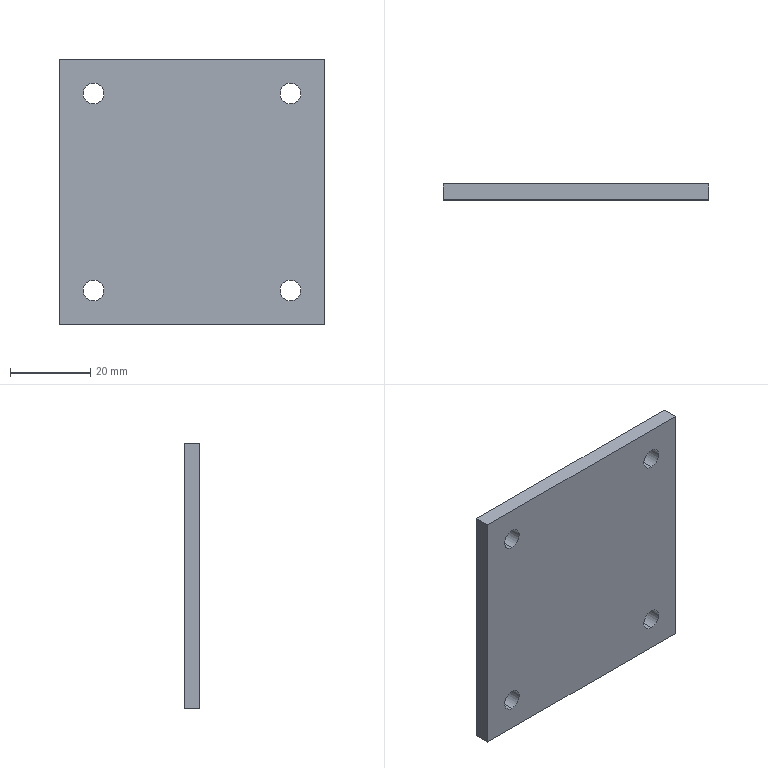Part | STEP file | 1 solid | 14 faces | box 66.15 x 3.92 x 66.15 mm | volume 16827 mm3 | cylinder 8 | plane 6 | commonest cylinder face diameters 5.145 x8
STEP:
#1=CARTESIAN_POINT('',(0.,0.,0.));
#2=DIRECTION('',(0.,0.,1.));
#3=DIRECTION('',(1.,0.,0.));
#4=AXIS2_PLACEMENT_3D('',#1,#2,#3);
#5=CARTESIAN_POINT('',(925.539,-111.474,188.835));
#6=VERTEX_POINT('',#5);
#7=CARTESIAN_POINT('',(925.539,-111.474,183.69));
#8=VERTEX_POINT('',#7);
#9=CARTESIAN_POINT('',(925.539,-111.474,186.262));
#10=DIRECTION('',(0.,1.,0.));
#11=DIRECTION('',(0.,0.,1.));
#12=AXIS2_PLACEMENT_3D('',#9,#10,#11);
#13=CIRCLE('',#12,2.572);
#14=CARTESIAN_POINT('',(925.539,-111.474,186.262));
#15=DIRECTION('',(0.,1.,0.));
#16=DIRECTION('',(0.,0.,1.));
#17=AXIS2_PLACEMENT_3D('',#14,#15,#16);
#18=CYLINDRICAL_SURFACE('',#17,2.572);
#19=CARTESIAN_POINT('',(0.,0.));
#20=DIRECTION('',(1.,0.));
#21=VECTOR('',#20,1.);
#22=LINE('',#19,#21);
#23=(GEOMETRIC_REPRESENTATION_CONTEXT(2)PARAMETRIC_REPRESENTATION_CONTEXT()REPRESENTATION_CONTEXT('',''));
#24=DEFINITIONAL_REPRESENTATION('',(#22),#23);
#25=PCURVE('',#18,#24);
#26=CARTESIAN_POINT('',(983.114,-111.474,194.837));
#27=DIRECTION('',(0.,1.,0.));
#28=DIRECTION('',(1.,0.,0.));
#29=AXIS2_PLACEMENT_3D('',#26,#27,#28);
#30=PLANE('',#29);
#31=CARTESIAN_POINT('',(-57.575,8.575));
#32=DIRECTION('',(0.,-1.));
#33=AXIS2_PLACEMENT_2D('',#31,#32);
#34=CIRCLE('',#33,2.572);
#35=(GEOMETRIC_REPRESENTATION_CONTEXT(2)PARAMETRIC_REPRESENTATION_CONTEXT()REPRESENTATION_CONTEXT('',''));
#36=DEFINITIONAL_REPRESENTATION('',(#34),#35);
#37=PCURVE('',#30,#36);
#38=SURFACE_CURVE('',#13,(#25,#37),.PCURVE_S1.);
#39=EDGE_CURVE('',#6,#8,#38,.T.);
#40=ORIENTED_EDGE('',*,*,#39,.F.);
#41=CARTESIAN_POINT('',(925.539,-115.394,188.835));
#42=VERTEX_POINT('',#41);
#43=CARTESIAN_POINT('',(925.539,-111.474,188.835));
#44=DIRECTION('',(0.,1.,0.));
#45=VECTOR('',#44,1.);
#46=LINE('',#43,#45);
#47=CARTESIAN_POINT('',(0.,0.));
#48=DIRECTION('',(0.,1.));
#49=VECTOR('',#48,1.);
#50=LINE('',#47,#49);
#51=(GEOMETRIC_REPRESENTATION_CONTEXT(2)PARAMETRIC_REPRESENTATION_CONTEXT()REPRESENTATION_CONTEXT('',''));
#52=DEFINITIONAL_REPRESENTATION('',(#50),#51);
#53=PCURVE('',#18,#52);
#54=CARTESIAN_POINT('',(925.539,-111.474,186.262));
#55=DIRECTION('',(0.,1.,0.));
#56=DIRECTION('',(0.,0.,1.));
#57=AXIS2_PLACEMENT_3D('',#54,#55,#56);
#58=CYLINDRICAL_SURFACE('',#57,2.572);
#59=CARTESIAN_POINT('',(6.283,0.));
#60=DIRECTION('',(0.,1.));
#61=VECTOR('',#60,1.);
#62=LINE('',#59,#61);
#63=(GEOMETRIC_REPRESENTATION_CONTEXT(2)PARAMETRIC_REPRESENTATION_CONTEXT()REPRESENTATION_CONTEXT('',''));
#64=DEFINITIONAL_REPRESENTATION('',(#62),#63);
#65=PCURVE('',#58,#64);
#66=SURFACE_CURVE('',#46,(#53,#65),.PCURVE_S1.);
#67=EDGE_CURVE('',#42,#6,#66,.T.);
#68=ORIENTED_EDGE('',*,*,#67,.F.);
#69=CARTESIAN_POINT('',(925.539,-115.394,183.69));
#70=VERTEX_POINT('',#69);
#71=CARTESIAN_POINT('',(925.539,-115.394,186.262));
#72=DIRECTION('',(0.,1.,0.));
#73=DIRECTION('',(0.,0.,1.));
#74=AXIS2_PLACEMENT_3D('',#71,#72,#73);
#75=CIRCLE('',#74,2.572);
#76=CARTESIAN_POINT('',(0.,-3.92));
#77=DIRECTION('',(1.,0.));
#78=VECTOR('',#77,1.);
#79=LINE('',#76,#78);
#80=(GEOMETRIC_REPRESENTATION_CONTEXT(2)PARAMETRIC_REPRESENTATION_CONTEXT()REPRESENTATION_CONTEXT('',''));
#81=DEFINITIONAL_REPRESENTATION('',(#79),#80);
#82=PCURVE('',#18,#81);
#83=CARTESIAN_POINT('',(983.114,-115.394,194.837));
#84=DIRECTION('',(0.,1.,0.));
#85=DIRECTION('',(1.,0.,0.));
#86=AXIS2_PLACEMENT_3D('',#83,#84,#85);
#87=PLANE('',#86);
#88=CARTESIAN_POINT('',(-57.575,8.575));
#89=DIRECTION('',(0.,-1.));
#90=AXIS2_PLACEMENT_2D('',#88,#89);
#91=CIRCLE('',#90,2.572);
#92=(GEOMETRIC_REPRESENTATION_CONTEXT(2)PARAMETRIC_REPRESENTATION_CONTEXT()REPRESENTATION_CONTEXT('',''));
#93=DEFINITIONAL_REPRESENTATION('',(#91),#92);
#94=PCURVE('',#87,#93);
#95=SURFACE_CURVE('',#75,(#82,#94),.PCURVE_S1.);
#96=EDGE_CURVE('',#42,#70,#95,.T.);
#97=ORIENTED_EDGE('',*,*,#96,.T.);
#98=CARTESIAN_POINT('',(925.539,-111.474,183.69));
#99=DIRECTION('',(0.,1.,0.));
#100=VECTOR('',#99,1.);
#101=LINE('',#98,#100);
#102=CARTESIAN_POINT('',(3.142,0.));
#103=DIRECTION('',(0.,1.));
#104=VECTOR('',#103,1.);
#105=LINE('',#102,#104);
#106=(GEOMETRIC_REPRESENTATION_CONTEXT(2)PARAMETRIC_REPRESENTATION_CONTEXT()REPRESENTATION_CONTEXT('',''));
#107=DEFINITIONAL_REPRESENTATION('',(#105),#106);
#108=PCURVE('',#18,#107);
#109=CARTESIAN_POINT('',(3.142,0.));
#110=DIRECTION('',(0.,1.));
#111=VECTOR('',#110,1.);
#112=LINE('',#109,#111);
#113=(GEOMETRIC_REPRESENTATION_CONTEXT(2)PARAMETRIC_REPRESENTATION_CONTEXT()REPRESENTATION_CONTEXT('',''));
#114=DEFINITIONAL_REPRESENTATION('',(#112),#113);
#115=PCURVE('',#58,#114);
#116=SURFACE_CURVE('',#101,(#108,#115),.PCURVE_S1.);
#117=EDGE_CURVE('',#70,#8,#116,.T.);
#118=ORIENTED_EDGE('',*,*,#117,.T.);
#119=EDGE_LOOP('',(#40,#68,#97,#118));
#120=FACE_BOUND('',#119,.F.);
#121=ADVANCED_FACE('',(#120),#18,.F.);
#122=CARTESIAN_POINT('',(974.539,-111.474,188.835));
#123=VERTEX_POINT('',#122);
#124=CARTESIAN_POINT('',(974.539,-111.474,183.69));
#125=VERTEX_POINT('',#124);
#126=CARTESIAN_POINT('',(974.539,-111.474,186.262));
#127=DIRECTION('',(0.,1.,0.));
#128=DIRECTION('',(0.,0.,1.));
#129=AXIS2_PLACEMENT_3D('',#126,#127,#128);
#130=CIRCLE('',#129,2.572);
#131=CARTESIAN_POINT('',(974.539,-111.474,186.262));
#132=DIRECTION('',(0.,1.,0.));
#133=DIRECTION('',(0.,0.,1.));
#134=AXIS2_PLACEMENT_3D('',#131,#132,#133);
#135=CYLINDRICAL_SURFACE('',#134,2.572);
#136=CARTESIAN_POINT('',(0.,0.));
#137=DIRECTION('',(1.,0.));
#138=VECTOR('',#137,1.);
#139=LINE('',#136,#138);
#140=(GEOMETRIC_REPRESENTATION_CONTEXT(2)PARAMETRIC_REPRESENTATION_CONTEXT()REPRESENTATION_CONTEXT('',''));
#141=DEFINITIONAL_REPRESENTATION('',(#139),#140);
#142=PCURVE('',#135,#141);
#143=CARTESIAN_POINT('',(-8.575,8.575));
#144=DIRECTION('',(0.,-1.));
#145=AXIS2_PLACEMENT_2D('',#143,#144);
#146=CIRCLE('',#145,2.572);
#147=(GEOMETRIC_REPRESENTATION_CONTEXT(2)PARAMETRIC_REPRESENTATION_CONTEXT()REPRESENTATION_CONTEXT('',''));
#148=DEFINITIONAL_REPRESENTATION('',(#146),#147);
#149=PCURVE('',#30,#148);
#150=SURFACE_CURVE('',#130,(#142,#149),.PCURVE_S1.);
#151=EDGE_CURVE('',#123,#125,#150,.T.);
#152=ORIENTED_EDGE('',*,*,#151,.F.);
#153=CARTESIAN_POINT('',(974.539,-115.394,188.835));
#154=VERTEX_POINT('',#153);
#155=CARTESIAN_POINT('',(974.539,-111.474,188.835));
#156=DIRECTION('',(0.,1.,0.));
#157=VECTOR('',#156,1.);
#158=LINE('',#155,#157);
#159=CARTESIAN_POINT('',(0.,0.));
#160=DIRECTION('',(0.,1.));
#161=VECTOR('',#160,1.);
#162=LINE('',#159,#161);
#163=(GEOMETRIC_REPRESENTATION_CONTEXT(2)PARAMETRIC_REPRESENTATION_CONTEXT()REPRESENTATION_CONTEXT('',''));
#164=DEFINITIONAL_REPRESENTATION('',(#162),#163);
#165=PCURVE('',#135,#164);
#166=CARTESIAN_POINT('',(974.539,-111.474,186.262));
#167=DIRECTION('',(0.,1.,0.));
#168=DIRECTION('',(0.,0.,1.));
#169=AXIS2_PLACEMENT_3D('',#166,#167,#168);
#170=CYLINDRICAL_SURFACE('',#169,2.572);
#171=CARTESIAN_POINT('',(6.283,0.));
#172=DIRECTION('',(0.,1.));
#173=VECTOR('',#172,1.);
#174=LINE('',#171,#173);
#175=(GEOMETRIC_REPRESENTATION_CONTEXT(2)PARAMETRIC_REPRESENTATION_CONTEXT()REPRESENTATION_CONTEXT('',''));
#176=DEFINITIONAL_REPRESENTATION('',(#174),#175);
#177=PCURVE('',#170,#176);
#178=SURFACE_CURVE('',#158,(#165,#177),.PCURVE_S1.);
#179=EDGE_CURVE('',#154,#123,#178,.T.);
#180=ORIENTED_EDGE('',*,*,#179,.F.);
#181=CARTESIAN_POINT('',(974.539,-115.394,183.69));
#182=VERTEX_POINT('',#181);
#183=CARTESIAN_POINT('',(974.539,-115.394,186.262));
#184=DIRECTION('',(0.,1.,0.));
#185=DIRECTION('',(0.,0.,1.));
#186=AXIS2_PLACEMENT_3D('',#183,#184,#185);
#187=CIRCLE('',#186,2.572);
#188=CARTESIAN_POINT('',(0.,-3.92));
#189=DIRECTION('',(1.,0.));
#190=VECTOR('',#189,1.);
#191=LINE('',#188,#190);
#192=(GEOMETRIC_REPRESENTATION_CONTEXT(2)PARAMETRIC_REPRESENTATION_CONTEXT()REPRESENTATION_CONTEXT('',''));
#193=DEFINITIONAL_REPRESENTATION('',(#191),#192);
#194=PCURVE('',#135,#193);
#195=CARTESIAN_POINT('',(-8.575,8.575));
#196=DIRECTION('',(0.,-1.));
#197=AXIS2_PLACEMENT_2D('',#195,#196);
#198=CIRCLE('',#197,2.572);
#199=(GEOMETRIC_REPRESENTATION_CONTEXT(2)PARAMETRIC_REPRESENTATION_CONTEXT()REPRESENTATION_CONTEXT('',''));
#200=DEFINITIONAL_REPRESENTATION('',(#198),#199);
#201=PCURVE('',#87,#200);
#202=SURFACE_CURVE('',#187,(#194,#201),.PCURVE_S1.);
#203=EDGE_CURVE('',#154,#182,#202,.T.);
#204=ORIENTED_EDGE('',*,*,#203,.T.);
#205=CARTESIAN_POINT('',(974.539,-111.474,183.69));
#206=DIRECTION('',(0.,1.,0.));
#207=VECTOR('',#206,1.);
#208=LINE('',#205,#207);
#209=CARTESIAN_POINT('',(3.142,0.));
#210=DIRECTION('',(0.,1.));
#211=VECTOR('',#210,1.);
#212=LINE('',#209,#211);
#213=(GEOMETRIC_REPRESENTATION_CONTEXT(2)PARAMETRIC_REPRESENTATION_CONTEXT()REPRESENTATION_CONTEXT('',''));
#214=DEFINITIONAL_REPRESENTATION('',(#212),#213);
#215=PCURVE('',#135,#214);
#216=CARTESIAN_POINT('',(3.142,0.));
#217=DIRECTION('',(0.,1.));
#218=VECTOR('',#217,1.);
#219=LINE('',#216,#218);
#220=(GEOMETRIC_REPRESENTATION_CONTEXT(2)PARAMETRIC_REPRESENTATION_CONTEXT()REPRESENTATION_CONTEXT('',''));
#221=DEFINITIONAL_REPRESENTATION('',(#219),#220);
#222=PCURVE('',#170,#221);
#223=SURFACE_CURVE('',#208,(#215,#222),.PCURVE_S1.);
#224=EDGE_CURVE('',#182,#125,#223,.T.);
#225=ORIENTED_EDGE('',*,*,#224,.T.);
#226=EDGE_LOOP('',(#152,#180,#204,#225));
#227=FACE_BOUND('',#226,.F.);
#228=ADVANCED_FACE('',(#227),#135,.F.);
#229=CARTESIAN_POINT('',(916.964,-115.394,194.837));
#230=VERTEX_POINT('',#229);
#231=CARTESIAN_POINT('',(916.964,-115.394,128.687));
#232=VERTEX_POINT('',#231);
#233=CARTESIAN_POINT('',(916.964,-115.394,194.837));
#234=DIRECTION('',(0.,0.,-1.));
#235=VECTOR('',#234,1.);
#236=LINE('',#233,#235);
#237=CARTESIAN_POINT('',(916.964,-111.474,161.762));
#238=DIRECTION('',(-1.,0.,0.));
#239=DIRECTION('',(0.,0.,1.));
#240=AXIS2_PLACEMENT_3D('',#237,#238,#239);
#241=PLANE('',#240);
#242=CARTESIAN_POINT('',(33.075,-3.92));
#243=DIRECTION('',(-1.,0.));
#244=VECTOR('',#243,1.);
#245=LINE('',#242,#244);
#246=(GEOMETRIC_REPRESENTATION_CONTEXT(2)PARAMETRIC_REPRESENTATION_CONTEXT()REPRESENTATION_CONTEXT('',''));
#247=DEFINITIONAL_REPRESENTATION('',(#245),#246);
#248=PCURVE('',#241,#247);
#249=CARTESIAN_POINT('',(-66.15,0.));
#250=DIRECTION('',(0.,1.));
#251=VECTOR('',#250,1.);
#252=LINE('',#249,#251);
#253=(GEOMETRIC_REPRESENTATION_CONTEXT(2)PARAMETRIC_REPRESENTATION_CONTEXT()REPRESENTATION_CONTEXT('',''));
#254=DEFINITIONAL_REPRESENTATION('',(#252),#253);
#255=PCURVE('',#87,#254);
#256=SURFACE_CURVE('',#236,(#248,#255),.PCURVE_S1.);
#257=EDGE_CURVE('',#230,#232,#256,.T.);
#258=ORIENTED_EDGE('',*,*,#257,.F.);
#259=CARTESIAN_POINT('',(916.964,-111.474,194.837));
#260=VERTEX_POINT('',#259);
#261=CARTESIAN_POINT('',(916.964,-115.394,194.837));
#262=DIRECTION('',(0.,1.,0.));
#263=VECTOR('',#262,1.);
#264=LINE('',#261,#263);
#265=CARTESIAN_POINT('',(33.075,-3.92));
#266=DIRECTION('',(0.,1.));
#267=VECTOR('',#266,1.);
#268=LINE('',#265,#267);
#269=(GEOMETRIC_REPRESENTATION_CONTEXT(2)PARAMETRIC_REPRESENTATION_CONTEXT()REPRESENTATION_CONTEXT('',''));
#270=DEFINITIONAL_REPRESENTATION('',(#268),#269);
#271=PCURVE('',#241,#270);
#272=CARTESIAN_POINT('',(983.114,-115.394,194.837));
#273=DIRECTION('',(0.,0.,1.));
#274=DIRECTION('',(1.,0.,0.));
#275=AXIS2_PLACEMENT_3D('',#272,#273,#274);
#276=PLANE('',#275);
#277=CARTESIAN_POINT('',(-66.15,0.));
#278=DIRECTION('',(0.,1.));
#279=VECTOR('',#278,1.);
#280=LINE('',#277,#279);
#281=(GEOMETRIC_REPRESENTATION_CONTEXT(2)PARAMETRIC_REPRESENTATION_CONTEXT()REPRESENTATION_CONTEXT('',''));
#282=DEFINITIONAL_REPRESENTATION('',(#280),#281);
#283=PCURVE('',#276,#282);
#284=SURFACE_CURVE('',#264,(#271,#283),.PCURVE_S1.);
#285=EDGE_CURVE('',#230,#260,#284,.T.);
#286=ORIENTED_EDGE('',*,*,#285,.T.);
#287=CARTESIAN_POINT('',(916.964,-111.474,128.687));
#288=VERTEX_POINT('',#287);
#289=CARTESIAN_POINT('',(916.964,-111.474,194.837));
#290=DIRECTION('',(0.,0.,-1.));
#291=VECTOR('',#290,1.);
#292=LINE('',#289,#291);
#293=CARTESIAN_POINT('',(33.075,0.));
#294=DIRECTION('',(-1.,0.));
#295=VECTOR('',#294,1.);
#296=LINE('',#293,#295);
#297=(GEOMETRIC_REPRESENTATION_CONTEXT(2)PARAMETRIC_REPRESENTATION_CONTEXT()REPRESENTATION_CONTEXT('',''));
#298=DEFINITIONAL_REPRESENTATION('',(#296),#297);
#299=PCURVE('',#241,#298);
#300=CARTESIAN_POINT('',(-66.15,0.));
#301=DIRECTION('',(0.,1.));
#302=VECTOR('',#301,1.);
#303=LINE('',#300,#302);
#304=(GEOMETRIC_REPRESENTATION_CONTEXT(2)PARAMETRIC_REPRESENTATION_CONTEXT()REPRESENTATION_CONTEXT('',''));
#305=DEFINITIONAL_REPRESENTATION('',(#303),#304);
#306=PCURVE('',#30,#305);
#307=SURFACE_CURVE('',#292,(#299,#306),.PCURVE_S1.);
#308=EDGE_CURVE('',#260,#288,#307,.T.);
#309=ORIENTED_EDGE('',*,*,#308,.T.);
#310=CARTESIAN_POINT('',(916.964,-111.474,128.687));
#311=DIRECTION('',(0.,-1.,0.));
#312=VECTOR('',#311,1.);
#313=LINE('',#310,#312);
#314=CARTESIAN_POINT('',(-33.075,0.));
#315=DIRECTION('',(0.,-1.));
#316=VECTOR('',#315,1.);
#317=LINE('',#314,#316);
#318=(GEOMETRIC_REPRESENTATION_CONTEXT(2)PARAMETRIC_REPRESENTATION_CONTEXT()REPRESENTATION_CONTEXT('',''));
#319=DEFINITIONAL_REPRESENTATION('',(#317),#318);
#320=PCURVE('',#241,#319);
#321=CARTESIAN_POINT('',(983.114,-111.474,128.687));
#322=DIRECTION('',(0.,0.,-1.));
#323=DIRECTION('',(0.,-1.,0.));
#324=AXIS2_PLACEMENT_3D('',#321,#322,#323);
#325=PLANE('',#324);
#326=CARTESIAN_POINT('',(0.,66.15));
#327=DIRECTION('',(1.,0.));
#328=VECTOR('',#327,1.);
#329=LINE('',#326,#328);
#330=(GEOMETRIC_REPRESENTATION_CONTEXT(2)PARAMETRIC_REPRESENTATION_CONTEXT()REPRESENTATION_CONTEXT('',''));
#331=DEFINITIONAL_REPRESENTATION('',(#329),#330);
#332=PCURVE('',#325,#331);
#333=SURFACE_CURVE('',#313,(#320,#332),.PCURVE_S1.);
#334=EDGE_CURVE('',#288,#232,#333,.T.);
#335=ORIENTED_EDGE('',*,*,#334,.T.);
#336=EDGE_LOOP('',(#258,#286,#309,#335));
#337=FACE_BOUND('',#336,.T.);
#338=ADVANCED_FACE('',(#337),#241,.T.);
#339=CARTESIAN_POINT('',(983.114,-115.394,194.837));
#340=VERTEX_POINT('',#339);
#341=CARTESIAN_POINT('',(983.114,-115.394,128.687));
#342=VERTEX_POINT('',#341);
#343=CARTESIAN_POINT('',(983.114,-115.394,194.837));
#344=DIRECTION('',(0.,0.,-1.));
#345=VECTOR('',#344,1.);
#346=LINE('',#343,#345);
#347=CARTESIAN_POINT('',(983.114,-111.474,161.762));
#348=DIRECTION('',(-1.,0.,0.));
#349=DIRECTION('',(0.,0.,1.));
#350=AXIS2_PLACEMENT_3D('',#347,#348,#349);
#351=PLANE('',#350);
#352=CARTESIAN_POINT('',(33.075,-3.92));
#353=DIRECTION('',(-1.,0.));
#354=VECTOR('',#353,1.);
#355=LINE('',#352,#354);
#356=(GEOMETRIC_REPRESENTATION_CONTEXT(2)PARAMETRIC_REPRESENTATION_CONTEXT()REPRESENTATION_CONTEXT('',''));
#357=DEFINITIONAL_REPRESENTATION('',(#355),#356);
#358=PCURVE('',#351,#357);
#359=CARTESIAN_POINT('',(0.,0.));
#360=DIRECTION('',(0.,1.));
#361=VECTOR('',#360,1.);
#362=LINE('',#359,#361);
#363=(GEOMETRIC_REPRESENTATION_CONTEXT(2)PARAMETRIC_REPRESENTATION_CONTEXT()REPRESENTATION_CONTEXT('',''));
#364=DEFINITIONAL_REPRESENTATION('',(#362),#363);
#365=PCURVE('',#87,#364);
#366=SURFACE_CURVE('',#346,(#358,#365),.PCURVE_S1.);
#367=EDGE_CURVE('',#340,#342,#366,.T.);
#368=ORIENTED_EDGE('',*,*,#367,.T.);
#369=CARTESIAN_POINT('',(983.114,-111.474,128.687));
#370=VERTEX_POINT('',#369);
#371=CARTESIAN_POINT('',(983.114,-111.474,128.687));
#372=DIRECTION('',(0.,-1.,0.));
#373=VECTOR('',#372,1.);
#374=LINE('',#371,#373);
#375=CARTESIAN_POINT('',(-33.075,0.));
#376=DIRECTION('',(0.,-1.));
#377=VECTOR('',#376,1.);
#378=LINE('',#375,#377);
#379=(GEOMETRIC_REPRESENTATION_CONTEXT(2)PARAMETRIC_REPRESENTATION_CONTEXT()REPRESENTATION_CONTEXT('',''));
#380=DEFINITIONAL_REPRESENTATION('',(#378),#379);
#381=PCURVE('',#351,#380);
#382=CARTESIAN_POINT('',(0.,0.));
#383=DIRECTION('',(1.,0.));
#384=VECTOR('',#383,1.);
#385=LINE('',#382,#384);
#386=(GEOMETRIC_REPRESENTATION_CONTEXT(2)PARAMETRIC_REPRESENTATION_CONTEXT()REPRESENTATION_CONTEXT('',''));
#387=DEFINITIONAL_REPRESENTATION('',(#385),#386);
#388=PCURVE('',#325,#387);
#389=SURFACE_CURVE('',#374,(#381,#388),.PCURVE_S1.);
#390=EDGE_CURVE('',#370,#342,#389,.T.);
#391=ORIENTED_EDGE('',*,*,#390,.F.);
#392=CARTESIAN_POINT('',(983.114,-111.474,194.837));
#393=VERTEX_POINT('',#392);
#394=CARTESIAN_POINT('',(983.114,-111.474,194.837));
#395=DIRECTION('',(0.,0.,-1.));
#396=VECTOR('',#395,1.);
#397=LINE('',#394,#396);
#398=CARTESIAN_POINT('',(33.075,0.));
#399=DIRECTION('',(-1.,0.));
#400=VECTOR('',#399,1.);
#401=LINE('',#398,#400);
#402=(GEOMETRIC_REPRESENTATION_CONTEXT(2)PARAMETRIC_REPRESENTATION_CONTEXT()REPRESENTATION_CONTEXT('',''));
#403=DEFINITIONAL_REPRESENTATION('',(#401),#402);
#404=PCURVE('',#351,#403);
#405=CARTESIAN_POINT('',(0.,0.));
#406=DIRECTION('',(0.,1.));
#407=VECTOR('',#406,1.);
#408=LINE('',#405,#407);
#409=(GEOMETRIC_REPRESENTATION_CONTEXT(2)PARAMETRIC_REPRESENTATION_CONTEXT()REPRESENTATION_CONTEXT('',''));
#410=DEFINITIONAL_REPRESENTATION('',(#408),#409);
#411=PCURVE('',#30,#410);
#412=SURFACE_CURVE('',#397,(#404,#411),.PCURVE_S1.);
#413=EDGE_CURVE('',#393,#370,#412,.T.);
#414=ORIENTED_EDGE('',*,*,#413,.F.);
#415=CARTESIAN_POINT('',(983.114,-115.394,194.837));
#416=DIRECTION('',(0.,1.,0.));
#417=VECTOR('',#416,1.);
#418=LINE('',#415,#417);
#419=CARTESIAN_POINT('',(33.075,-3.92));
#420=DIRECTION('',(0.,1.));
#421=VECTOR('',#420,1.);
#422=LINE('',#419,#421);
#423=(GEOMETRIC_REPRESENTATION_CONTEXT(2)PARAMETRIC_REPRESENTATION_CONTEXT()REPRESENTATION_CONTEXT('',''));
#424=DEFINITIONAL_REPRESENTATION('',(#422),#423);
#425=PCURVE('',#351,#424);
#426=CARTESIAN_POINT('',(0.,0.));
#427=DIRECTION('',(0.,1.));
#428=VECTOR('',#427,1.);
#429=LINE('',#426,#428);
#430=(GEOMETRIC_REPRESENTATION_CONTEXT(2)PARAMETRIC_REPRESENTATION_CONTEXT()REPRESENTATION_CONTEXT('',''));
#431=DEFINITIONAL_REPRESENTATION('',(#429),#430);
#432=PCURVE('',#276,#431);
#433=SURFACE_CURVE('',#418,(#425,#432),.PCURVE_S1.);
#434=EDGE_CURVE('',#340,#393,#433,.T.);
#435=ORIENTED_EDGE('',*,*,#434,.F.);
#436=EDGE_LOOP('',(#368,#391,#414,#435));
#437=FACE_BOUND('',#436,.T.);
#438=ADVANCED_FACE('',(#437),#351,.F.);
#439=ORIENTED_EDGE('',*,*,#285,.F.);
#440=CARTESIAN_POINT('',(983.114,-115.394,194.837));
#441=DIRECTION('',(-1.,0.,0.));
#442=VECTOR('',#441,1.);
#443=LINE('',#440,#442);
#444=CARTESIAN_POINT('',(0.,0.));
#445=DIRECTION('',(-1.,0.));
#446=VECTOR('',#445,1.);
#447=LINE('',#444,#446);
#448=(GEOMETRIC_REPRESENTATION_CONTEXT(2)PARAMETRIC_REPRESENTATION_CONTEXT()REPRESENTATION_CONTEXT('',''));
#449=DEFINITIONAL_REPRESENTATION('',(#447),#448);
#450=PCURVE('',#276,#449);
#451=CARTESIAN_POINT('',(0.,0.));
#452=DIRECTION('',(-1.,0.));
#453=VECTOR('',#452,1.);
#454=LINE('',#451,#453);
#455=(GEOMETRIC_REPRESENTATION_CONTEXT(2)PARAMETRIC_REPRESENTATION_CONTEXT()REPRESENTATION_CONTEXT('',''));
#456=DEFINITIONAL_REPRESENTATION('',(#454),#455);
#457=PCURVE('',#87,#456);
#458=SURFACE_CURVE('',#443,(#450,#457),.PCURVE_S1.);
#459=EDGE_CURVE('',#340,#230,#458,.T.);
#460=ORIENTED_EDGE('',*,*,#459,.F.);
#461=ORIENTED_EDGE('',*,*,#434,.T.);
#462=CARTESIAN_POINT('',(983.114,-111.474,194.837));
#463=DIRECTION('',(-1.,0.,0.));
#464=VECTOR('',#463,1.);
#465=LINE('',#462,#464);
#466=CARTESIAN_POINT('',(0.,3.92));
#467=DIRECTION('',(-1.,0.));
#468=VECTOR('',#467,1.);
#469=LINE('',#466,#468);
#470=(GEOMETRIC_REPRESENTATION_CONTEXT(2)PARAMETRIC_REPRESENTATION_CONTEXT()REPRESENTATION_CONTEXT('',''));
#471=DEFINITIONAL_REPRESENTATION('',(#469),#470);
#472=PCURVE('',#276,#471);
#473=CARTESIAN_POINT('',(0.,0.));
#474=DIRECTION('',(-1.,0.));
#475=VECTOR('',#474,1.);
#476=LINE('',#473,#475);
#477=(GEOMETRIC_REPRESENTATION_CONTEXT(2)PARAMETRIC_REPRESENTATION_CONTEXT()REPRESENTATION_CONTEXT('',''));
#478=DEFINITIONAL_REPRESENTATION('',(#476),#477);
#479=PCURVE('',#30,#478);
#480=SURFACE_CURVE('',#465,(#472,#479),.PCURVE_S1.);
#481=EDGE_CURVE('',#393,#260,#480,.T.);
#482=ORIENTED_EDGE('',*,*,#481,.T.);
#483=EDGE_LOOP('',(#439,#460,#461,#482));
#484=FACE_BOUND('',#483,.T.);
#485=ADVANCED_FACE('',(#484),#276,.T.);
#486=CARTESIAN_POINT('',(925.539,-111.474,139.835));
#487=VERTEX_POINT('',#486);
#488=CARTESIAN_POINT('',(925.539,-111.474,134.69));
#489=VERTEX_POINT('',#488);
#490=CARTESIAN_POINT('',(925.539,-111.474,137.262));
#491=DIRECTION('',(0.,1.,0.));
#492=DIRECTION('',(0.,0.,1.));
#493=AXIS2_PLACEMENT_3D('',#490,#491,#492);
#494=CIRCLE('',#493,2.572);
#495=CARTESIAN_POINT('',(-57.575,57.575));
#496=DIRECTION('',(0.,-1.));
#497=AXIS2_PLACEMENT_2D('',#495,#496);
#498=CIRCLE('',#497,2.572);
#499=(GEOMETRIC_REPRESENTATION_CONTEXT(2)PARAMETRIC_REPRESENTATION_CONTEXT()REPRESENTATION_CONTEXT('',''));
#500=DEFINITIONAL_REPRESENTATION('',(#498),#499);
#501=PCURVE('',#30,#500);
#502=CARTESIAN_POINT('',(925.539,-111.474,137.262));
#503=DIRECTION('',(0.,1.,0.));
#504=DIRECTION('',(0.,0.,1.));
#505=AXIS2_PLACEMENT_3D('',#502,#503,#504);
#506=CYLINDRICAL_SURFACE('',#505,2.572);
#507=CARTESIAN_POINT('',(0.,0.));
#508=DIRECTION('',(1.,0.));
#509=VECTOR('',#508,1.);
#510=LINE('',#507,#509);
#511=(GEOMETRIC_REPRESENTATION_CONTEXT(2)PARAMETRIC_REPRESENTATION_CONTEXT()REPRESENTATION_CONTEXT('',''));
#512=DEFINITIONAL_REPRESENTATION('',(#510),#511);
#513=PCURVE('',#506,#512);
#514=SURFACE_CURVE('',#494,(#501,#513),.PCURVE_S1.);
#515=EDGE_CURVE('',#487,#489,#514,.T.);
#516=ORIENTED_EDGE('',*,*,#515,.F.);
#517=CARTESIAN_POINT('',(925.539,-111.474,137.262));
#518=DIRECTION('',(0.,1.,0.));
#519=DIRECTION('',(0.,0.,1.));
#520=AXIS2_PLACEMENT_3D('',#517,#518,#519);
#521=CIRCLE('',#520,2.572);
#522=CARTESIAN_POINT('',(-57.575,57.575));
#523=DIRECTION('',(0.,-1.));
#524=AXIS2_PLACEMENT_2D('',#522,#523);
#525=CIRCLE('',#524,2.572);
#526=(GEOMETRIC_REPRESENTATION_CONTEXT(2)PARAMETRIC_REPRESENTATION_CONTEXT()REPRESENTATION_CONTEXT('',''));
#527=DEFINITIONAL_REPRESENTATION('',(#525),#526);
#528=PCURVE('',#30,#527);
#529=CARTESIAN_POINT('',(925.539,-111.474,137.262));
#530=DIRECTION('',(0.,1.,0.));
#531=DIRECTION('',(0.,0.,1.));
#532=AXIS2_PLACEMENT_3D('',#529,#530,#531);
#533=CYLINDRICAL_SURFACE('',#532,2.572);
#534=CARTESIAN_POINT('',(0.,0.));
#535=DIRECTION('',(1.,0.));
#536=VECTOR('',#535,1.);
#537=LINE('',#534,#536);
#538=(GEOMETRIC_REPRESENTATION_CONTEXT(2)PARAMETRIC_REPRESENTATION_CONTEXT()REPRESENTATION_CONTEXT('',''));
#539=DEFINITIONAL_REPRESENTATION('',(#537),#538);
#540=PCURVE('',#533,#539);
#541=SURFACE_CURVE('',#521,(#528,#540),.PCURVE_S1.);
#542=EDGE_CURVE('',#489,#487,#541,.T.);
#543=ORIENTED_EDGE('',*,*,#542,.F.);
#544=EDGE_LOOP('',(#516,#543));
#545=FACE_BOUND('',#544,.T.);
#546=CARTESIAN_POINT('',(974.539,-111.474,139.835));
#547=VERTEX_POINT('',#546);
#548=CARTESIAN_POINT('',(974.539,-111.474,134.69));
#549=VERTEX_POINT('',#548);
#550=CARTESIAN_POINT('',(974.539,-111.474,137.262));
#551=DIRECTION('',(0.,1.,0.));
#552=DIRECTION('',(0.,0.,1.));
#553=AXIS2_PLACEMENT_3D('',#550,#551,#552);
#554=CIRCLE('',#553,2.572);
#555=CARTESIAN_POINT('',(-8.575,57.575));
#556=DIRECTION('',(0.,-1.));
#557=AXIS2_PLACEMENT_2D('',#555,#556);
#558=CIRCLE('',#557,2.572);
#559=(GEOMETRIC_REPRESENTATION_CONTEXT(2)PARAMETRIC_REPRESENTATION_CONTEXT()REPRESENTATION_CONTEXT('',''));
#560=DEFINITIONAL_REPRESENTATION('',(#558),#559);
#561=PCURVE('',#30,#560);
#562=CARTESIAN_POINT('',(974.539,-111.474,137.262));
#563=DIRECTION('',(0.,1.,0.));
#564=DIRECTION('',(0.,0.,1.));
#565=AXIS2_PLACEMENT_3D('',#562,#563,#564);
#566=CYLINDRICAL_SURFACE('',#565,2.572);
#567=CARTESIAN_POINT('',(0.,0.));
#568=DIRECTION('',(1.,0.));
#569=VECTOR('',#568,1.);
#570=LINE('',#567,#569);
#571=(GEOMETRIC_REPRESENTATION_CONTEXT(2)PARAMETRIC_REPRESENTATION_CONTEXT()REPRESENTATION_CONTEXT('',''));
#572=DEFINITIONAL_REPRESENTATION('',(#570),#571);
#573=PCURVE('',#566,#572);
#574=SURFACE_CURVE('',#554,(#561,#573),.PCURVE_S1.);
#575=EDGE_CURVE('',#547,#549,#574,.T.);
#576=ORIENTED_EDGE('',*,*,#575,.F.);
#577=CARTESIAN_POINT('',(974.539,-111.474,137.262));
#578=DIRECTION('',(0.,1.,0.));
#579=DIRECTION('',(0.,0.,1.));
#580=AXIS2_PLACEMENT_3D('',#577,#578,#579);
#581=CIRCLE('',#580,2.572);
#582=CARTESIAN_POINT('',(-8.575,57.575));
#583=DIRECTION('',(0.,-1.));
#584=AXIS2_PLACEMENT_2D('',#582,#583);
#585=CIRCLE('',#584,2.572);
#586=(GEOMETRIC_REPRESENTATION_CONTEXT(2)PARAMETRIC_REPRESENTATION_CONTEXT()REPRESENTATION_CONTEXT('',''));
#587=DEFINITIONAL_REPRESENTATION('',(#585),#586);
#588=PCURVE('',#30,#587);
#589=CARTESIAN_POINT('',(974.539,-111.474,137.262));
#590=DIRECTION('',(0.,1.,0.));
#591=DIRECTION('',(0.,0.,1.));
#592=AXIS2_PLACEMENT_3D('',#589,#590,#591);
#593=CYLINDRICAL_SURFACE('',#592,2.572);
#594=CARTESIAN_POINT('',(0.,0.));
#595=DIRECTION('',(1.,0.));
#596=VECTOR('',#595,1.);
#597=LINE('',#594,#596);
#598=(GEOMETRIC_REPRESENTATION_CONTEXT(2)PARAMETRIC_REPRESENTATION_CONTEXT()REPRESENTATION_CONTEXT('',''));
#599=DEFINITIONAL_REPRESENTATION('',(#597),#598);
#600=PCURVE('',#593,#599);
#601=SURFACE_CURVE('',#581,(#588,#600),.PCURVE_S1.);
#602=EDGE_CURVE('',#549,#547,#601,.T.);
#603=ORIENTED_EDGE('',*,*,#602,.F.);
#604=EDGE_LOOP('',(#576,#603));
#605=FACE_BOUND('',#604,.T.);
#606=ORIENTED_EDGE('',*,*,#151,.F.);
#607=CARTESIAN_POINT('',(974.539,-111.474,186.262));
#608=DIRECTION('',(0.,1.,0.));
#609=DIRECTION('',(0.,0.,1.));
#610=AXIS2_PLACEMENT_3D('',#607,#608,#609);
#611=CIRCLE('',#610,2.572);
#612=CARTESIAN_POINT('',(-8.575,8.575));
#613=DIRECTION('',(0.,-1.));
#614=AXIS2_PLACEMENT_2D('',#612,#613);
#615=CIRCLE('',#614,2.572);
#616=(GEOMETRIC_REPRESENTATION_CONTEXT(2)PARAMETRIC_REPRESENTATION_CONTEXT()REPRESENTATION_CONTEXT('',''));
#617=DEFINITIONAL_REPRESENTATION('',(#615),#616);
#618=PCURVE('',#30,#617);
#619=CARTESIAN_POINT('',(0.,0.));
#620=DIRECTION('',(1.,0.));
#621=VECTOR('',#620,1.);
#622=LINE('',#619,#621);
#623=(GEOMETRIC_REPRESENTATION_CONTEXT(2)PARAMETRIC_REPRESENTATION_CONTEXT()REPRESENTATION_CONTEXT('',''));
#624=DEFINITIONAL_REPRESENTATION('',(#622),#623);
#625=PCURVE('',#170,#624);
#626=SURFACE_CURVE('',#611,(#618,#625),.PCURVE_S1.);
#627=EDGE_CURVE('',#125,#123,#626,.T.);
#628=ORIENTED_EDGE('',*,*,#627,.F.);
#629=EDGE_LOOP('',(#606,#628));
#630=FACE_BOUND('',#629,.T.);
#631=ORIENTED_EDGE('',*,*,#39,.F.);
#632=CARTESIAN_POINT('',(925.539,-111.474,186.262));
#633=DIRECTION('',(0.,1.,0.));
#634=DIRECTION('',(0.,0.,1.));
#635=AXIS2_PLACEMENT_3D('',#632,#633,#634);
#636=CIRCLE('',#635,2.572);
#637=CARTESIAN_POINT('',(-57.575,8.575));
#638=DIRECTION('',(0.,-1.));
#639=AXIS2_PLACEMENT_2D('',#637,#638);
#640=CIRCLE('',#639,2.572);
#641=(GEOMETRIC_REPRESENTATION_CONTEXT(2)PARAMETRIC_REPRESENTATION_CONTEXT()REPRESENTATION_CONTEXT('',''));
#642=DEFINITIONAL_REPRESENTATION('',(#640),#641);
#643=PCURVE('',#30,#642);
#644=CARTESIAN_POINT('',(0.,0.));
#645=DIRECTION('',(1.,0.));
#646=VECTOR('',#645,1.);
#647=LINE('',#644,#646);
#648=(GEOMETRIC_REPRESENTATION_CONTEXT(2)PARAMETRIC_REPRESENTATION_CONTEXT()REPRESENTATION_CONTEXT('',''));
#649=DEFINITIONAL_REPRESENTATION('',(#647),#648);
#650=PCURVE('',#58,#649);
#651=SURFACE_CURVE('',#636,(#643,#650),.PCURVE_S1.);
#652=EDGE_CURVE('',#8,#6,#651,.T.);
#653=ORIENTED_EDGE('',*,*,#652,.F.);
#654=EDGE_LOOP('',(#631,#653));
#655=FACE_BOUND('',#654,.T.);
#656=ORIENTED_EDGE('',*,*,#308,.F.);
#657=ORIENTED_EDGE('',*,*,#481,.F.);
#658=ORIENTED_EDGE('',*,*,#413,.T.);
#659=CARTESIAN_POINT('',(983.114,-111.474,128.687));
#660=DIRECTION('',(-1.,0.,0.));
#661=VECTOR('',#660,1.);
#662=LINE('',#659,#661);
#663=CARTESIAN_POINT('',(0.,66.15));
#664=DIRECTION('',(-1.,0.));
#665=VECTOR('',#664,1.);
#666=LINE('',#663,#665);
#667=(GEOMETRIC_REPRESENTATION_CONTEXT(2)PARAMETRIC_REPRESENTATION_CONTEXT()REPRESENTATION_CONTEXT('',''));
#668=DEFINITIONAL_REPRESENTATION('',(#666),#667);
#669=PCURVE('',#30,#668);
#670=CARTESIAN_POINT('',(0.,0.));
#671=DIRECTION('',(0.,1.));
#672=VECTOR('',#671,1.);
#673=LINE('',#670,#672);
#674=(GEOMETRIC_REPRESENTATION_CONTEXT(2)PARAMETRIC_REPRESENTATION_CONTEXT()REPRESENTATION_CONTEXT('',''));
#675=DEFINITIONAL_REPRESENTATION('',(#673),#674);
#676=PCURVE('',#325,#675);
#677=SURFACE_CURVE('',#662,(#669,#676),.PCURVE_S1.);
#678=EDGE_CURVE('',#370,#288,#677,.T.);
#679=ORIENTED_EDGE('',*,*,#678,.T.);
#680=EDGE_LOOP('',(#656,#657,#658,#679));
#681=FACE_BOUND('',#680,.T.);
#682=ADVANCED_FACE('',(#545,#605,#630,#655,#681),#30,.T.);
#683=ORIENTED_EDGE('',*,*,#334,.F.);
#684=ORIENTED_EDGE('',*,*,#678,.F.);
#685=ORIENTED_EDGE('',*,*,#390,.T.);
#686=CARTESIAN_POINT('',(983.114,-115.394,128.687));
#687=DIRECTION('',(-1.,0.,0.));
#688=VECTOR('',#687,1.);
#689=LINE('',#686,#688);
#690=CARTESIAN_POINT('',(3.92,0.));
#691=DIRECTION('',(0.,1.));
#692=VECTOR('',#691,1.);
#693=LINE('',#690,#692);
#694=(GEOMETRIC_REPRESENTATION_CONTEXT(2)PARAMETRIC_REPRESENTATION_CONTEXT()REPRESENTATION_CONTEXT('',''));
#695=DEFINITIONAL_REPRESENTATION('',(#693),#694);
#696=PCURVE('',#325,#695);
#697=CARTESIAN_POINT('',(0.,66.15));
#698=DIRECTION('',(-1.,0.));
#699=VECTOR('',#698,1.);
#700=LINE('',#697,#699);
#701=(GEOMETRIC_REPRESENTATION_CONTEXT(2)PARAMETRIC_REPRESENTATION_CONTEXT()REPRESENTATION_CONTEXT('',''));
#702=DEFINITIONAL_REPRESENTATION('',(#700),#701);
#703=PCURVE('',#87,#702);
#704=SURFACE_CURVE('',#689,(#696,#703),.PCURVE_S1.);
#705=EDGE_CURVE('',#342,#232,#704,.T.);
#706=ORIENTED_EDGE('',*,*,#705,.T.);
#707=EDGE_LOOP('',(#683,#684,#685,#706));
#708=FACE_BOUND('',#707,.T.);
#709=ADVANCED_FACE('',(#708),#325,.T.);
#710=CARTESIAN_POINT('',(925.539,-115.394,139.835));
#711=VERTEX_POINT('',#710);
#712=CARTESIAN_POINT('',(925.539,-115.394,134.69));
#713=VERTEX_POINT('',#712);
#714=CARTESIAN_POINT('',(925.539,-115.394,137.262));
#715=DIRECTION('',(0.,1.,0.));
#716=DIRECTION('',(0.,0.,1.));
#717=AXIS2_PLACEMENT_3D('',#714,#715,#716);
#718=CIRCLE('',#717,2.572);
#719=CARTESIAN_POINT('',(-57.575,57.575));
#720=DIRECTION('',(0.,-1.));
#721=AXIS2_PLACEMENT_2D('',#719,#720);
#722=CIRCLE('',#721,2.572);
#723=(GEOMETRIC_REPRESENTATION_CONTEXT(2)PARAMETRIC_REPRESENTATION_CONTEXT()REPRESENTATION_CONTEXT('',''));
#724=DEFINITIONAL_REPRESENTATION('',(#722),#723);
#725=PCURVE('',#87,#724);
#726=CARTESIAN_POINT('',(0.,-3.92));
#727=DIRECTION('',(1.,0.));
#728=VECTOR('',#727,1.);
#729=LINE('',#726,#728);
#730=(GEOMETRIC_REPRESENTATION_CONTEXT(2)PARAMETRIC_REPRESENTATION_CONTEXT()REPRESENTATION_CONTEXT('',''));
#731=DEFINITIONAL_REPRESENTATION('',(#729),#730);
#732=PCURVE('',#506,#731);
#733=SURFACE_CURVE('',#718,(#725,#732),.PCURVE_S1.);
#734=EDGE_CURVE('',#711,#713,#733,.T.);
#735=ORIENTED_EDGE('',*,*,#734,.T.);
#736=CARTESIAN_POINT('',(925.539,-115.394,137.262));
#737=DIRECTION('',(0.,1.,0.));
#738=DIRECTION('',(0.,0.,1.));
#739=AXIS2_PLACEMENT_3D('',#736,#737,#738);
#740=CIRCLE('',#739,2.572);
#741=CARTESIAN_POINT('',(-57.575,57.575));
#742=DIRECTION('',(0.,-1.));
#743=AXIS2_PLACEMENT_2D('',#741,#742);
#744=CIRCLE('',#743,2.572);
#745=(GEOMETRIC_REPRESENTATION_CONTEXT(2)PARAMETRIC_REPRESENTATION_CONTEXT()REPRESENTATION_CONTEXT('',''));
#746=DEFINITIONAL_REPRESENTATION('',(#744),#745);
#747=PCURVE('',#87,#746);
#748=CARTESIAN_POINT('',(0.,-3.92));
#749=DIRECTION('',(1.,0.));
#750=VECTOR('',#749,1.);
#751=LINE('',#748,#750);
#752=(GEOMETRIC_REPRESENTATION_CONTEXT(2)PARAMETRIC_REPRESENTATION_CONTEXT()REPRESENTATION_CONTEXT('',''));
#753=DEFINITIONAL_REPRESENTATION('',(#751),#752);
#754=PCURVE('',#533,#753);
#755=SURFACE_CURVE('',#740,(#747,#754),.PCURVE_S1.);
#756=EDGE_CURVE('',#713,#711,#755,.T.);
#757=ORIENTED_EDGE('',*,*,#756,.T.);
#758=EDGE_LOOP('',(#735,#757));
#759=FACE_BOUND('',#758,.T.);
#760=CARTESIAN_POINT('',(974.539,-115.394,139.835));
#761=VERTEX_POINT('',#760);
#762=CARTESIAN_POINT('',(974.539,-115.394,134.69));
#763=VERTEX_POINT('',#762);
#764=CARTESIAN_POINT('',(974.539,-115.394,137.262));
#765=DIRECTION('',(0.,1.,0.));
#766=DIRECTION('',(0.,0.,1.));
#767=AXIS2_PLACEMENT_3D('',#764,#765,#766);
#768=CIRCLE('',#767,2.572);
#769=CARTESIAN_POINT('',(-8.575,57.575));
#770=DIRECTION('',(0.,-1.));
#771=AXIS2_PLACEMENT_2D('',#769,#770);
#772=CIRCLE('',#771,2.572);
#773=(GEOMETRIC_REPRESENTATION_CONTEXT(2)PARAMETRIC_REPRESENTATION_CONTEXT()REPRESENTATION_CONTEXT('',''));
#774=DEFINITIONAL_REPRESENTATION('',(#772),#773);
#775=PCURVE('',#87,#774);
#776=CARTESIAN_POINT('',(0.,-3.92));
#777=DIRECTION('',(1.,0.));
#778=VECTOR('',#777,1.);
#779=LINE('',#776,#778);
#780=(GEOMETRIC_REPRESENTATION_CONTEXT(2)PARAMETRIC_REPRESENTATION_CONTEXT()REPRESENTATION_CONTEXT('',''));
#781=DEFINITIONAL_REPRESENTATION('',(#779),#780);
#782=PCURVE('',#566,#781);
#783=SURFACE_CURVE('',#768,(#775,#782),.PCURVE_S1.);
#784=EDGE_CURVE('',#761,#763,#783,.T.);
#785=ORIENTED_EDGE('',*,*,#784,.T.);
#786=CARTESIAN_POINT('',(974.539,-115.394,137.262));
#787=DIRECTION('',(0.,1.,0.));
#788=DIRECTION('',(0.,0.,1.));
#789=AXIS2_PLACEMENT_3D('',#786,#787,#788);
#790=CIRCLE('',#789,2.572);
#791=CARTESIAN_POINT('',(-8.575,57.575));
#792=DIRECTION('',(0.,-1.));
#793=AXIS2_PLACEMENT_2D('',#791,#792);
#794=CIRCLE('',#793,2.572);
#795=(GEOMETRIC_REPRESENTATION_CONTEXT(2)PARAMETRIC_REPRESENTATION_CONTEXT()REPRESENTATION_CONTEXT('',''));
#796=DEFINITIONAL_REPRESENTATION('',(#794),#795);
#797=PCURVE('',#87,#796);
#798=CARTESIAN_POINT('',(0.,-3.92));
#799=DIRECTION('',(1.,0.));
#800=VECTOR('',#799,1.);
#801=LINE('',#798,#800);
#802=(GEOMETRIC_REPRESENTATION_CONTEXT(2)PARAMETRIC_REPRESENTATION_CONTEXT()REPRESENTATION_CONTEXT('',''));
#803=DEFINITIONAL_REPRESENTATION('',(#801),#802);
#804=PCURVE('',#593,#803);
#805=SURFACE_CURVE('',#790,(#797,#804),.PCURVE_S1.);
#806=EDGE_CURVE('',#763,#761,#805,.T.);
#807=ORIENTED_EDGE('',*,*,#806,.T.);
#808=EDGE_LOOP('',(#785,#807));
#809=FACE_BOUND('',#808,.T.);
#810=ORIENTED_EDGE('',*,*,#203,.T.);
#811=CARTESIAN_POINT('',(974.539,-115.394,186.262));
#812=DIRECTION('',(0.,1.,0.));
#813=DIRECTION('',(0.,0.,1.));
#814=AXIS2_PLACEMENT_3D('',#811,#812,#813);
#815=CIRCLE('',#814,2.572);
#816=CARTESIAN_POINT('',(-8.575,8.575));
#817=DIRECTION('',(0.,-1.));
#818=AXIS2_PLACEMENT_2D('',#816,#817);
#819=CIRCLE('',#818,2.572);
#820=(GEOMETRIC_REPRESENTATION_CONTEXT(2)PARAMETRIC_REPRESENTATION_CONTEXT()REPRESENTATION_CONTEXT('',''));
#821=DEFINITIONAL_REPRESENTATION('',(#819),#820);
#822=PCURVE('',#87,#821);
#823=CARTESIAN_POINT('',(0.,-3.92));
#824=DIRECTION('',(1.,0.));
#825=VECTOR('',#824,1.);
#826=LINE('',#823,#825);
#827=(GEOMETRIC_REPRESENTATION_CONTEXT(2)PARAMETRIC_REPRESENTATION_CONTEXT()REPRESENTATION_CONTEXT('',''));
#828=DEFINITIONAL_REPRESENTATION('',(#826),#827);
#829=PCURVE('',#170,#828);
#830=SURFACE_CURVE('',#815,(#822,#829),.PCURVE_S1.);
#831=EDGE_CURVE('',#182,#154,#830,.T.);
#832=ORIENTED_EDGE('',*,*,#831,.T.);
#833=EDGE_LOOP('',(#810,#832));
#834=FACE_BOUND('',#833,.T.);
#835=ORIENTED_EDGE('',*,*,#96,.T.);
#836=CARTESIAN_POINT('',(925.539,-115.394,186.262));
#837=DIRECTION('',(0.,1.,0.));
#838=DIRECTION('',(0.,0.,1.));
#839=AXIS2_PLACEMENT_3D('',#836,#837,#838);
#840=CIRCLE('',#839,2.572);
#841=CARTESIAN_POINT('',(-57.575,8.575));
#842=DIRECTION('',(0.,-1.));
#843=AXIS2_PLACEMENT_2D('',#841,#842);
#844=CIRCLE('',#843,2.572);
#845=(GEOMETRIC_REPRESENTATION_CONTEXT(2)PARAMETRIC_REPRESENTATION_CONTEXT()REPRESENTATION_CONTEXT('',''));
#846=DEFINITIONAL_REPRESENTATION('',(#844),#845);
#847=PCURVE('',#87,#846);
#848=CARTESIAN_POINT('',(0.,-3.92));
#849=DIRECTION('',(1.,0.));
#850=VECTOR('',#849,1.);
#851=LINE('',#848,#850);
#852=(GEOMETRIC_REPRESENTATION_CONTEXT(2)PARAMETRIC_REPRESENTATION_CONTEXT()REPRESENTATION_CONTEXT('',''));
#853=DEFINITIONAL_REPRESENTATION('',(#851),#852);
#854=PCURVE('',#58,#853);
#855=SURFACE_CURVE('',#840,(#847,#854),.PCURVE_S1.);
#856=EDGE_CURVE('',#70,#42,#855,.T.);
#857=ORIENTED_EDGE('',*,*,#856,.T.);
#858=EDGE_LOOP('',(#835,#857));
#859=FACE_BOUND('',#858,.T.);
#860=ORIENTED_EDGE('',*,*,#257,.T.);
#861=ORIENTED_EDGE('',*,*,#705,.F.);
#862=ORIENTED_EDGE('',*,*,#367,.F.);
#863=ORIENTED_EDGE('',*,*,#459,.T.);
#864=EDGE_LOOP('',(#860,#861,#862,#863));
#865=FACE_BOUND('',#864,.T.);
#866=ADVANCED_FACE('',(#759,#809,#834,#859,#865),#87,.F.);
#867=ORIENTED_EDGE('',*,*,#575,.F.);
#868=CARTESIAN_POINT('',(974.539,-111.474,139.835));
#869=DIRECTION('',(0.,1.,0.));
#870=VECTOR('',#869,1.);
#871=LINE('',#868,#870);
#872=CARTESIAN_POINT('',(0.,0.));
#873=DIRECTION('',(0.,1.));
#874=VECTOR('',#873,1.);
#875=LINE('',#872,#874);
#876=(GEOMETRIC_REPRESENTATION_CONTEXT(2)PARAMETRIC_REPRESENTATION_CONTEXT()REPRESENTATION_CONTEXT('',''));
#877=DEFINITIONAL_REPRESENTATION('',(#875),#876);
#878=PCURVE('',#566,#877);
#879=CARTESIAN_POINT('',(6.283,0.));
#880=DIRECTION('',(0.,1.));
#881=VECTOR('',#880,1.);
#882=LINE('',#879,#881);
#883=(GEOMETRIC_REPRESENTATION_CONTEXT(2)PARAMETRIC_REPRESENTATION_CONTEXT()REPRESENTATION_CONTEXT('',''));
#884=DEFINITIONAL_REPRESENTATION('',(#882),#883);
#885=PCURVE('',#593,#884);
#886=SURFACE_CURVE('',#871,(#878,#885),.PCURVE_S1.);
#887=EDGE_CURVE('',#761,#547,#886,.T.);
#888=ORIENTED_EDGE('',*,*,#887,.F.);
#889=ORIENTED_EDGE('',*,*,#784,.T.);
#890=CARTESIAN_POINT('',(974.539,-111.474,134.69));
#891=DIRECTION('',(0.,1.,0.));
#892=VECTOR('',#891,1.);
#893=LINE('',#890,#892);
#894=CARTESIAN_POINT('',(3.142,0.));
#895=DIRECTION('',(0.,1.));
#896=VECTOR('',#895,1.);
#897=LINE('',#894,#896);
#898=(GEOMETRIC_REPRESENTATION_CONTEXT(2)PARAMETRIC_REPRESENTATION_CONTEXT()REPRESENTATION_CONTEXT('',''));
#899=DEFINITIONAL_REPRESENTATION('',(#897),#898);
#900=PCURVE('',#566,#899);
#901=CARTESIAN_POINT('',(3.142,0.));
#902=DIRECTION('',(0.,1.));
#903=VECTOR('',#902,1.);
#904=LINE('',#901,#903);
#905=(GEOMETRIC_REPRESENTATION_CONTEXT(2)PARAMETRIC_REPRESENTATION_CONTEXT()REPRESENTATION_CONTEXT('',''));
#906=DEFINITIONAL_REPRESENTATION('',(#904),#905);
#907=PCURVE('',#593,#906);
#908=SURFACE_CURVE('',#893,(#900,#907),.PCURVE_S1.);
#909=EDGE_CURVE('',#763,#549,#908,.T.);
#910=ORIENTED_EDGE('',*,*,#909,.T.);
#911=EDGE_LOOP('',(#867,#888,#889,#910));
#912=FACE_BOUND('',#911,.F.);
#913=ADVANCED_FACE('',(#912),#566,.F.);
#914=ORIENTED_EDGE('',*,*,#515,.F.);
#915=CARTESIAN_POINT('',(925.539,-111.474,139.835));
#916=DIRECTION('',(0.,1.,0.));
#917=VECTOR('',#916,1.);
#918=LINE('',#915,#917);
#919=CARTESIAN_POINT('',(0.,0.));
#920=DIRECTION('',(0.,1.));
#921=VECTOR('',#920,1.);
#922=LINE('',#919,#921);
#923=(GEOMETRIC_REPRESENTATION_CONTEXT(2)PARAMETRIC_REPRESENTATION_CONTEXT()REPRESENTATION_CONTEXT('',''));
#924=DEFINITIONAL_REPRESENTATION('',(#922),#923);
#925=PCURVE('',#506,#924);
#926=CARTESIAN_POINT('',(6.283,0.));
#927=DIRECTION('',(0.,1.));
#928=VECTOR('',#927,1.);
#929=LINE('',#926,#928);
#930=(GEOMETRIC_REPRESENTATION_CONTEXT(2)PARAMETRIC_REPRESENTATION_CONTEXT()REPRESENTATION_CONTEXT('',''));
#931=DEFINITIONAL_REPRESENTATION('',(#929),#930);
#932=PCURVE('',#533,#931);
#933=SURFACE_CURVE('',#918,(#925,#932),.PCURVE_S1.);
#934=EDGE_CURVE('',#711,#487,#933,.T.);
#935=ORIENTED_EDGE('',*,*,#934,.F.);
#936=ORIENTED_EDGE('',*,*,#734,.T.);
#937=CARTESIAN_POINT('',(925.539,-111.474,134.69));
#938=DIRECTION('',(0.,1.,0.));
#939=VECTOR('',#938,1.);
#940=LINE('',#937,#939);
#941=CARTESIAN_POINT('',(3.142,0.));
#942=DIRECTION('',(0.,1.));
#943=VECTOR('',#942,1.);
#944=LINE('',#941,#943);
#945=(GEOMETRIC_REPRESENTATION_CONTEXT(2)PARAMETRIC_REPRESENTATION_CONTEXT()REPRESENTATION_CONTEXT('',''));
#946=DEFINITIONAL_REPRESENTATION('',(#944),#945);
#947=PCURVE('',#506,#946);
#948=CARTESIAN_POINT('',(3.142,0.));
#949=DIRECTION('',(0.,1.));
#950=VECTOR('',#949,1.);
#951=LINE('',#948,#950);
#952=(GEOMETRIC_REPRESENTATION_CONTEXT(2)PARAMETRIC_REPRESENTATION_CONTEXT()REPRESENTATION_CONTEXT('',''));
#953=DEFINITIONAL_REPRESENTATION('',(#951),#952);
#954=PCURVE('',#533,#953);
#955=SURFACE_CURVE('',#940,(#947,#954),.PCURVE_S1.);
#956=EDGE_CURVE('',#713,#489,#955,.T.);
#957=ORIENTED_EDGE('',*,*,#956,.T.);
#958=EDGE_LOOP('',(#914,#935,#936,#957));
#959=FACE_BOUND('',#958,.F.);
#960=ADVANCED_FACE('',(#959),#506,.F.);
#961=ORIENTED_EDGE('',*,*,#934,.T.);
#962=ORIENTED_EDGE('',*,*,#542,.F.);
#963=ORIENTED_EDGE('',*,*,#956,.F.);
#964=ORIENTED_EDGE('',*,*,#756,.T.);
#965=EDGE_LOOP('',(#961,#962,#963,#964));
#966=FACE_BOUND('',#965,.F.);
#967=ADVANCED_FACE('',(#966),#533,.F.);
#968=ORIENTED_EDGE('',*,*,#887,.T.);
#969=ORIENTED_EDGE('',*,*,#602,.F.);
#970=ORIENTED_EDGE('',*,*,#909,.F.);
#971=ORIENTED_EDGE('',*,*,#806,.T.);
#972=EDGE_LOOP('',(#968,#969,#970,#971));
#973=FACE_BOUND('',#972,.F.);
#974=ADVANCED_FACE('',(#973),#593,.F.);
#975=ORIENTED_EDGE('',*,*,#179,.T.);
#976=ORIENTED_EDGE('',*,*,#627,.F.);
#977=ORIENTED_EDGE('',*,*,#224,.F.);
#978=ORIENTED_EDGE('',*,*,#831,.T.);
#979=EDGE_LOOP('',(#975,#976,#977,#978));
#980=FACE_BOUND('',#979,.F.);
#981=ADVANCED_FACE('',(#980),#170,.F.);
#982=ORIENTED_EDGE('',*,*,#67,.T.);
#983=ORIENTED_EDGE('',*,*,#652,.F.);
#984=ORIENTED_EDGE('',*,*,#117,.F.);
#985=ORIENTED_EDGE('',*,*,#856,.T.);
#986=EDGE_LOOP('',(#982,#983,#984,#985));
#987=FACE_BOUND('',#986,.F.);
#988=ADVANCED_FACE('',(#987),#58,.F.);
#989=CLOSED_SHELL('',(#121,#228,#338,#438,#485,#682,#709,#866,#913,#960,#967,#974,#981,#988));
#990=MANIFOLD_SOLID_BREP('',#989);
#991=(LENGTH_UNIT()NAMED_UNIT(*)SI_UNIT(.MILLI.,.METRE.));
#992=UNCERTAINTY_MEASURE_WITH_UNIT(LENGTH_MEASURE(0.0000001),#991,'','');
#993=(NAMED_UNIT(*)PLANE_ANGLE_UNIT()SI_UNIT($,.RADIAN.));
#994=(NAMED_UNIT(*)SI_UNIT($,.STERADIAN.)SOLID_ANGLE_UNIT());
#995=(GEOMETRIC_REPRESENTATION_CONTEXT(3)GLOBAL_UNCERTAINTY_ASSIGNED_CONTEXT((#992))GLOBAL_UNIT_ASSIGNED_CONTEXT((#991,#993,#994))REPRESENTATION_CONTEXT('',''));
#996=ADVANCED_BREP_SHAPE_REPRESENTATION('',(#4,#990),#995);